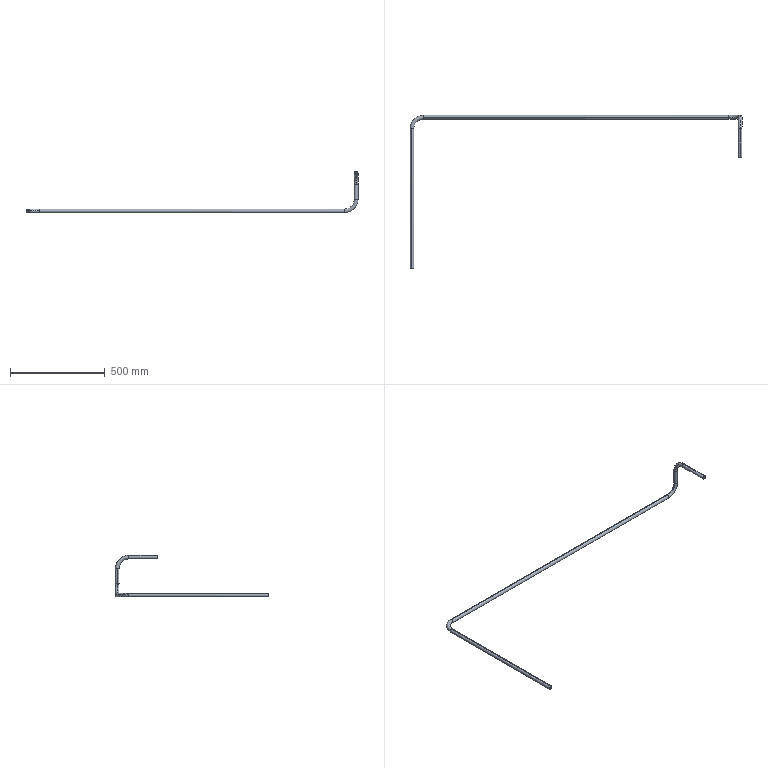Part | SolidWorks | features 3DProfileFeature 2, Sweep 1 | 1 solid | 30 faces | box 1755 x 810 x 220 mm | volume 676261 mm3 | cylinder 16 | torus 12 | plane 2 | commonest cylinder face diameters 10 x8 20 x8
STEP:
#1=CARTESIAN_POINT('',(725.349,1850.038,-1305.));
#2=VERTEX_POINT('',#1);
#3=CARTESIAN_POINT('',(725.349,1855.038,-1300.));
#4=VERTEX_POINT('',#3);
#5=CARTESIAN_POINT('',(725.349,1850.038,-1300.));
#6=DIRECTION('',(1.,0.,0.));
#7=DIRECTION('',(0.,0.,1.));
#8=AXIS2_PLACEMENT_3D('',#5,#6,#7);
#9=CIRCLE('',#8,5.);
#10=EDGE_CURVE('',#2,#4,#9,.T.);
#11=ORIENTED_EDGE('',*,*,#10,.T.);
#12=CARTESIAN_POINT('',(660.349,1790.038,-1300.));
#13=VERTEX_POINT('',#12);
#14=CARTESIAN_POINT('',(725.349,1790.038,-1300.));
#15=DIRECTION('',(0.,0.,1.));
#16=DIRECTION('',(1.,0.,0.));
#17=AXIS2_PLACEMENT_3D('',#14,#15,#16);
#18=CIRCLE('',#17,65.);
#19=EDGE_CURVE('',#4,#13,#18,.T.);
#20=ORIENTED_EDGE('',*,*,#19,.T.);
#21=CARTESIAN_POINT('',(665.349,1790.038,-1305.));
#22=VERTEX_POINT('',#21);
#23=CARTESIAN_POINT('',(665.349,1790.038,-1300.));
#24=DIRECTION('',(0.,1.,0.));
#25=DIRECTION('',(-1.,0.,0.));
#26=AXIS2_PLACEMENT_3D('',#23,#24,#25);
#27=CIRCLE('',#26,5.);
#28=EDGE_CURVE('',#22,#13,#27,.T.);
#29=ORIENTED_EDGE('',*,*,#28,.F.);
#30=CARTESIAN_POINT('',(670.349,1790.038,-1300.));
#31=VERTEX_POINT('',#30);
#32=CARTESIAN_POINT('',(665.349,1790.038,-1300.));
#33=DIRECTION('',(0.,1.,0.));
#34=DIRECTION('',(-1.,0.,0.));
#35=AXIS2_PLACEMENT_3D('',#32,#33,#34);
#36=CIRCLE('',#35,5.);
#37=EDGE_CURVE('',#31,#22,#36,.T.);
#38=ORIENTED_EDGE('',*,*,#37,.F.);
#39=CARTESIAN_POINT('',(725.349,1845.038,-1300.));
#40=VERTEX_POINT('',#39);
#41=CARTESIAN_POINT('',(725.349,1790.038,-1300.));
#42=DIRECTION('',(0.,0.,1.));
#43=DIRECTION('',(1.,0.,0.));
#44=AXIS2_PLACEMENT_3D('',#41,#42,#43);
#45=CIRCLE('',#44,55.);
#46=EDGE_CURVE('',#40,#31,#45,.T.);
#47=ORIENTED_EDGE('',*,*,#46,.F.);
#48=CARTESIAN_POINT('',(725.349,1850.038,-1300.));
#49=DIRECTION('',(1.,0.,0.));
#50=DIRECTION('',(0.,0.,1.));
#51=AXIS2_PLACEMENT_3D('',#48,#49,#50);
#52=CIRCLE('',#51,5.);
#53=EDGE_CURVE('',#40,#2,#52,.T.);
#54=ORIENTED_EDGE('',*,*,#53,.T.);
#55=EDGE_LOOP('',(#11,#20,#29,#38,#47,#54));
#56=FACE_OUTER_BOUND('',#55,.T.);
#57=CARTESIAN_POINT('',(725.349,1790.038,-1300.));
#58=DIRECTION('',(0.,0.,1.));
#59=DIRECTION('',(1.,0.,0.));
#60=AXIS2_PLACEMENT_3D('',#57,#58,#59);
#61=TOROIDAL_SURFACE('',#60,60.,5.);
#62=ADVANCED_FACE('',(#56),#61,.F.);
#63=CARTESIAN_POINT('',(2395.,1850.038,-1240.));
#64=VERTEX_POINT('',#63);
#65=CARTESIAN_POINT('',(2405.,1850.038,-1240.));
#66=VERTEX_POINT('',#65);
#67=CARTESIAN_POINT('',(2400.,1850.038,-1240.));
#68=DIRECTION('',(0.,0.,1.));
#69=DIRECTION('',(-1.,0.,0.));
#70=AXIS2_PLACEMENT_3D('',#67,#68,#69);
#71=CIRCLE('',#70,5.);
#72=EDGE_CURVE('',#64,#66,#71,.T.);
#73=ORIENTED_EDGE('',*,*,#72,.T.);
#74=CARTESIAN_POINT('',(2340.,1850.038,-1305.));
#75=VERTEX_POINT('',#74);
#76=CARTESIAN_POINT('',(2340.,1850.038,-1240.));
#77=DIRECTION('',(0.,1.,0.));
#78=DIRECTION('',(0.,0.,1.));
#79=AXIS2_PLACEMENT_3D('',#76,#77,#78);
#80=CIRCLE('',#79,65.);
#81=EDGE_CURVE('',#66,#75,#80,.T.);
#82=ORIENTED_EDGE('',*,*,#81,.T.);
#83=CARTESIAN_POINT('',(2340.,1850.038,-1295.));
#84=VERTEX_POINT('',#83);
#85=CARTESIAN_POINT('',(2340.,1850.038,-1300.));
#86=DIRECTION('',(1.,0.,0.));
#87=DIRECTION('',(0.,0.,-1.));
#88=AXIS2_PLACEMENT_3D('',#85,#86,#87);
#89=CIRCLE('',#88,5.);
#90=EDGE_CURVE('',#84,#75,#89,.T.);
#91=ORIENTED_EDGE('',*,*,#90,.F.);
#92=CARTESIAN_POINT('',(2340.,1850.038,-1240.));
#93=DIRECTION('',(0.,1.,0.));
#94=DIRECTION('',(0.,0.,1.));
#95=AXIS2_PLACEMENT_3D('',#92,#93,#94);
#96=CIRCLE('',#95,55.);
#97=EDGE_CURVE('',#64,#84,#96,.T.);
#98=ORIENTED_EDGE('',*,*,#97,.F.);
#99=EDGE_LOOP('',(#73,#82,#91,#98));
#100=FACE_OUTER_BOUND('',#99,.T.);
#101=CARTESIAN_POINT('',(2340.,1850.038,-1240.));
#102=DIRECTION('',(0.,1.,0.));
#103=DIRECTION('',(0.,0.,1.));
#104=AXIS2_PLACEMENT_3D('',#101,#102,#103);
#105=TOROIDAL_SURFACE('',#104,60.,5.);
#106=ADVANCED_FACE('',(#100),#105,.F.);
#107=CARTESIAN_POINT('',(2400.,1790.038,-1105.));
#108=VERTEX_POINT('',#107);
#109=CARTESIAN_POINT('',(2400.,1790.038,-1095.));
#110=VERTEX_POINT('',#109);
#111=CARTESIAN_POINT('',(2400.,1790.038,-1100.));
#112=DIRECTION('',(0.,-1.,0.));
#113=DIRECTION('',(0.,0.,1.));
#114=AXIS2_PLACEMENT_3D('',#111,#112,#113);
#115=CIRCLE('',#114,5.);
#116=EDGE_CURVE('',#108,#110,#115,.T.);
#117=ORIENTED_EDGE('',*,*,#116,.T.);
#118=CARTESIAN_POINT('',(2400.,1855.038,-1160.));
#119=VERTEX_POINT('',#118);
#120=CARTESIAN_POINT('',(2400.,1790.038,-1160.));
#121=DIRECTION('',(-1.,0.,0.));
#122=DIRECTION('',(0.,0.,1.));
#123=AXIS2_PLACEMENT_3D('',#120,#121,#122);
#124=CIRCLE('',#123,65.);
#125=EDGE_CURVE('',#110,#119,#124,.T.);
#126=ORIENTED_EDGE('',*,*,#125,.T.);
#127=CARTESIAN_POINT('',(2405.,1850.038,-1160.));
#128=VERTEX_POINT('',#127);
#129=CARTESIAN_POINT('',(2400.,1850.038,-1160.));
#130=DIRECTION('',(0.,0.,1.));
#131=DIRECTION('',(0.,-1.,0.));
#132=AXIS2_PLACEMENT_3D('',#129,#130,#131);
#133=CIRCLE('',#132,5.);
#134=EDGE_CURVE('',#128,#119,#133,.T.);
#135=ORIENTED_EDGE('',*,*,#134,.F.);
#136=CARTESIAN_POINT('',(2400.,1845.038,-1160.));
#137=VERTEX_POINT('',#136);
#138=CARTESIAN_POINT('',(2400.,1850.038,-1160.));
#139=DIRECTION('',(0.,0.,1.));
#140=DIRECTION('',(0.,-1.,0.));
#141=AXIS2_PLACEMENT_3D('',#138,#139,#140);
#142=CIRCLE('',#141,5.);
#143=EDGE_CURVE('',#137,#128,#142,.T.);
#144=ORIENTED_EDGE('',*,*,#143,.F.);
#145=CARTESIAN_POINT('',(2400.,1790.038,-1160.));
#146=DIRECTION('',(-1.,0.,0.));
#147=DIRECTION('',(0.,0.,1.));
#148=AXIS2_PLACEMENT_3D('',#145,#146,#147);
#149=CIRCLE('',#148,55.);
#150=EDGE_CURVE('',#108,#137,#149,.T.);
#151=ORIENTED_EDGE('',*,*,#150,.F.);
#152=EDGE_LOOP('',(#117,#126,#135,#144,#151));
#153=FACE_OUTER_BOUND('',#152,.T.);
#154=CARTESIAN_POINT('',(2400.,1790.038,-1160.));
#155=DIRECTION('',(-1.,0.,0.));
#156=DIRECTION('',(0.,0.,1.));
#157=AXIS2_PLACEMENT_3D('',#154,#155,#156);
#158=TOROIDAL_SURFACE('',#157,60.,5.);
#159=ADVANCED_FACE('',(#153),#158,.F.);
#160=CARTESIAN_POINT('',(725.349,1860.038,-1300.));
#161=VERTEX_POINT('',#160);
#162=CARTESIAN_POINT('',(725.349,1850.038,-1290.));
#163=VERTEX_POINT('',#162);
#164=CARTESIAN_POINT('',(725.349,1850.038,-1300.));
#165=DIRECTION('',(1.,0.,0.));
#166=DIRECTION('',(0.,0.,1.));
#167=AXIS2_PLACEMENT_3D('',#164,#165,#166);
#168=CIRCLE('',#167,10.);
#169=EDGE_CURVE('',#161,#163,#168,.T.);
#170=ORIENTED_EDGE('',*,*,#169,.F.);
#171=CARTESIAN_POINT('',(655.349,1790.038,-1300.));
#172=VERTEX_POINT('',#171);
#173=CARTESIAN_POINT('',(725.349,1790.038,-1300.));
#174=DIRECTION('',(0.,0.,1.));
#175=DIRECTION('',(1.,0.,0.));
#176=AXIS2_PLACEMENT_3D('',#173,#174,#175);
#177=CIRCLE('',#176,70.);
#178=EDGE_CURVE('',#161,#172,#177,.T.);
#179=ORIENTED_EDGE('',*,*,#178,.T.);
#180=CARTESIAN_POINT('',(665.349,1790.038,-1290.));
#181=VERTEX_POINT('',#180);
#182=CARTESIAN_POINT('',(665.349,1790.038,-1300.));
#183=DIRECTION('',(0.,1.,0.));
#184=DIRECTION('',(0.,0.,1.));
#185=AXIS2_PLACEMENT_3D('',#182,#183,#184);
#186=CIRCLE('',#185,10.);
#187=EDGE_CURVE('',#172,#181,#186,.T.);
#188=ORIENTED_EDGE('',*,*,#187,.T.);
#189=CARTESIAN_POINT('',(675.349,1790.038,-1300.));
#190=VERTEX_POINT('',#189);
#191=CARTESIAN_POINT('',(665.349,1790.038,-1300.));
#192=DIRECTION('',(0.,1.,0.));
#193=DIRECTION('',(0.,0.,1.));
#194=AXIS2_PLACEMENT_3D('',#191,#192,#193);
#195=CIRCLE('',#194,10.);
#196=EDGE_CURVE('',#181,#190,#195,.T.);
#197=ORIENTED_EDGE('',*,*,#196,.T.);
#198=CARTESIAN_POINT('',(725.349,1840.038,-1300.));
#199=VERTEX_POINT('',#198);
#200=CARTESIAN_POINT('',(725.349,1790.038,-1300.));
#201=DIRECTION('',(0.,0.,1.));
#202=DIRECTION('',(1.,0.,0.));
#203=AXIS2_PLACEMENT_3D('',#200,#201,#202);
#204=CIRCLE('',#203,50.);
#205=EDGE_CURVE('',#199,#190,#204,.T.);
#206=ORIENTED_EDGE('',*,*,#205,.F.);
#207=CARTESIAN_POINT('',(725.349,1850.038,-1300.));
#208=DIRECTION('',(1.,0.,0.));
#209=DIRECTION('',(0.,0.,1.));
#210=AXIS2_PLACEMENT_3D('',#207,#208,#209);
#211=CIRCLE('',#210,10.);
#212=EDGE_CURVE('',#163,#199,#211,.T.);
#213=ORIENTED_EDGE('',*,*,#212,.F.);
#214=EDGE_LOOP('',(#170,#179,#188,#197,#206,#213));
#215=FACE_OUTER_BOUND('',#214,.T.);
#216=CARTESIAN_POINT('',(725.349,1790.038,-1300.));
#217=DIRECTION('',(0.,0.,1.));
#218=DIRECTION('',(1.,0.,0.));
#219=AXIS2_PLACEMENT_3D('',#216,#217,#218);
#220=TOROIDAL_SURFACE('',#219,60.,10.);
#221=ADVANCED_FACE('',(#215),#220,.T.);
#222=CARTESIAN_POINT('',(2410.,1850.038,-1240.));
#223=VERTEX_POINT('',#222);
#224=CARTESIAN_POINT('',(2390.,1850.038,-1240.));
#225=VERTEX_POINT('',#224);
#226=CARTESIAN_POINT('',(2400.,1850.038,-1240.));
#227=DIRECTION('',(0.,0.,1.));
#228=DIRECTION('',(-1.,0.,0.));
#229=AXIS2_PLACEMENT_3D('',#226,#227,#228);
#230=CIRCLE('',#229,10.);
#231=EDGE_CURVE('',#223,#225,#230,.T.);
#232=ORIENTED_EDGE('',*,*,#231,.F.);
#233=CARTESIAN_POINT('',(2340.,1850.038,-1310.));
#234=VERTEX_POINT('',#233);
#235=CARTESIAN_POINT('',(2340.,1850.038,-1240.));
#236=DIRECTION('',(0.,1.,0.));
#237=DIRECTION('',(0.,0.,1.));
#238=AXIS2_PLACEMENT_3D('',#235,#236,#237);
#239=CIRCLE('',#238,70.);
#240=EDGE_CURVE('',#223,#234,#239,.T.);
#241=ORIENTED_EDGE('',*,*,#240,.T.);
#242=CARTESIAN_POINT('',(2340.,1850.038,-1290.));
#243=VERTEX_POINT('',#242);
#244=CARTESIAN_POINT('',(2340.,1850.038,-1300.));
#245=DIRECTION('',(1.,0.,0.));
#246=DIRECTION('',(0.,0.,1.));
#247=AXIS2_PLACEMENT_3D('',#244,#245,#246);
#248=CIRCLE('',#247,10.);
#249=EDGE_CURVE('',#234,#243,#248,.T.);
#250=ORIENTED_EDGE('',*,*,#249,.T.);
#251=CARTESIAN_POINT('',(2340.,1850.038,-1240.));
#252=DIRECTION('',(0.,1.,0.));
#253=DIRECTION('',(0.,0.,1.));
#254=AXIS2_PLACEMENT_3D('',#251,#252,#253);
#255=CIRCLE('',#254,50.);
#256=EDGE_CURVE('',#225,#243,#255,.T.);
#257=ORIENTED_EDGE('',*,*,#256,.F.);
#258=EDGE_LOOP('',(#232,#241,#250,#257));
#259=FACE_OUTER_BOUND('',#258,.T.);
#260=CARTESIAN_POINT('',(2340.,1850.038,-1240.));
#261=DIRECTION('',(0.,1.,0.));
#262=DIRECTION('',(0.,0.,1.));
#263=AXIS2_PLACEMENT_3D('',#260,#261,#262);
#264=TOROIDAL_SURFACE('',#263,60.,10.);
#265=ADVANCED_FACE('',(#259),#264,.T.);
#266=CARTESIAN_POINT('',(2400.,1790.038,-1090.));
#267=VERTEX_POINT('',#266);
#268=CARTESIAN_POINT('',(2400.,1790.038,-1110.));
#269=VERTEX_POINT('',#268);
#270=CARTESIAN_POINT('',(2400.,1790.038,-1100.));
#271=DIRECTION('',(0.,-1.,0.));
#272=DIRECTION('',(-1.,0.,0.));
#273=AXIS2_PLACEMENT_3D('',#270,#271,#272);
#274=CIRCLE('',#273,10.);
#275=EDGE_CURVE('',#267,#269,#274,.T.);
#276=ORIENTED_EDGE('',*,*,#275,.F.);
#277=CARTESIAN_POINT('',(2400.,1860.038,-1160.));
#278=VERTEX_POINT('',#277);
#279=CARTESIAN_POINT('',(2400.,1790.038,-1160.));
#280=DIRECTION('',(-1.,0.,0.));
#281=DIRECTION('',(0.,0.,1.));
#282=AXIS2_PLACEMENT_3D('',#279,#280,#281);
#283=CIRCLE('',#282,70.);
#284=EDGE_CURVE('',#267,#278,#283,.T.);
#285=ORIENTED_EDGE('',*,*,#284,.T.);
#286=CARTESIAN_POINT('',(2390.,1850.038,-1160.));
#287=VERTEX_POINT('',#286);
#288=CARTESIAN_POINT('',(2400.,1850.038,-1160.));
#289=DIRECTION('',(0.,0.,1.));
#290=DIRECTION('',(-1.,0.,0.));
#291=AXIS2_PLACEMENT_3D('',#288,#289,#290);
#292=CIRCLE('',#291,10.);
#293=EDGE_CURVE('',#278,#287,#292,.T.);
#294=ORIENTED_EDGE('',*,*,#293,.T.);
#295=CARTESIAN_POINT('',(2400.,1840.038,-1160.));
#296=VERTEX_POINT('',#295);
#297=CARTESIAN_POINT('',(2400.,1850.038,-1160.));
#298=DIRECTION('',(0.,0.,1.));
#299=DIRECTION('',(-1.,0.,0.));
#300=AXIS2_PLACEMENT_3D('',#297,#298,#299);
#301=CIRCLE('',#300,10.);
#302=EDGE_CURVE('',#287,#296,#301,.T.);
#303=ORIENTED_EDGE('',*,*,#302,.T.);
#304=CARTESIAN_POINT('',(2400.,1790.038,-1160.));
#305=DIRECTION('',(-1.,0.,0.));
#306=DIRECTION('',(0.,0.,1.));
#307=AXIS2_PLACEMENT_3D('',#304,#305,#306);
#308=CIRCLE('',#307,50.);
#309=EDGE_CURVE('',#269,#296,#308,.T.);
#310=ORIENTED_EDGE('',*,*,#309,.F.);
#311=EDGE_LOOP('',(#276,#285,#294,#303,#310));
#312=FACE_OUTER_BOUND('',#311,.T.);
#313=CARTESIAN_POINT('',(2400.,1790.038,-1160.));
#314=DIRECTION('',(-1.,0.,0.));
#315=DIRECTION('',(0.,0.,1.));
#316=AXIS2_PLACEMENT_3D('',#313,#314,#315);
#317=TOROIDAL_SURFACE('',#316,60.,10.);
#318=ADVANCED_FACE('',(#312),#317,.T.);
#319=ORIENTED_EDGE('',*,*,#28,.T.);
#320=CARTESIAN_POINT('',(665.349,1790.038,-1295.));
#321=VERTEX_POINT('',#320);
#322=CARTESIAN_POINT('',(665.349,1790.038,-1300.));
#323=DIRECTION('',(0.,1.,0.));
#324=DIRECTION('',(-1.,0.,0.));
#325=AXIS2_PLACEMENT_3D('',#322,#323,#324);
#326=CIRCLE('',#325,5.);
#327=EDGE_CURVE('',#13,#321,#326,.T.);
#328=ORIENTED_EDGE('',*,*,#327,.T.);
#329=CARTESIAN_POINT('',(665.349,1050.038,-1295.));
#330=VERTEX_POINT('',#329);
#331=CARTESIAN_POINT('',(665.349,1790.038,-1295.));
#332=DIRECTION('',(0.,-1.,0.));
#333=VECTOR('',#332,1000.);
#334=LINE('',#331,#333);
#335=EDGE_CURVE('',#321,#330,#334,.T.);
#336=ORIENTED_EDGE('',*,*,#335,.T.);
#337=CARTESIAN_POINT('',(665.349,1050.038,-1305.));
#338=VERTEX_POINT('',#337);
#339=CARTESIAN_POINT('',(665.349,1050.038,-1300.));
#340=DIRECTION('',(0.,1.,0.));
#341=DIRECTION('',(0.,0.,1.));
#342=AXIS2_PLACEMENT_3D('',#339,#340,#341);
#343=CIRCLE('',#342,5.);
#344=EDGE_CURVE('',#338,#330,#343,.T.);
#345=ORIENTED_EDGE('',*,*,#344,.F.);
#346=CARTESIAN_POINT('',(665.349,1790.038,-1305.));
#347=DIRECTION('',(0.,-1.,0.));
#348=VECTOR('',#347,1000.);
#349=LINE('',#346,#348);
#350=EDGE_CURVE('',#22,#338,#349,.T.);
#351=ORIENTED_EDGE('',*,*,#350,.F.);
#352=EDGE_LOOP('',(#319,#328,#336,#345,#351));
#353=FACE_OUTER_BOUND('',#352,.T.);
#354=CARTESIAN_POINT('',(665.349,1790.038,-1300.));
#355=DIRECTION('',(0.,-1.,0.));
#356=DIRECTION('',(0.,0.,-1.));
#357=AXIS2_PLACEMENT_3D('',#354,#355,#356);
#358=CYLINDRICAL_SURFACE('',#357,5.);
#359=ADVANCED_FACE('',(#353),#358,.F.);
#360=ORIENTED_EDGE('',*,*,#90,.T.);
#361=CARTESIAN_POINT('',(2340.,1850.038,-1305.));
#362=DIRECTION('',(-1.,0.,0.));
#363=VECTOR('',#362,1000.);
#364=LINE('',#361,#363);
#365=EDGE_CURVE('',#75,#2,#364,.T.);
#366=ORIENTED_EDGE('',*,*,#365,.T.);
#367=ORIENTED_EDGE('',*,*,#53,.F.);
#368=CARTESIAN_POINT('',(725.349,1850.038,-1295.));
#369=VERTEX_POINT('',#368);
#370=CARTESIAN_POINT('',(725.349,1850.038,-1300.));
#371=DIRECTION('',(1.,0.,0.));
#372=DIRECTION('',(0.,0.,1.));
#373=AXIS2_PLACEMENT_3D('',#370,#371,#372);
#374=CIRCLE('',#373,5.);
#375=EDGE_CURVE('',#369,#40,#374,.T.);
#376=ORIENTED_EDGE('',*,*,#375,.F.);
#377=CARTESIAN_POINT('',(2340.,1850.038,-1295.));
#378=DIRECTION('',(-1.,0.,0.));
#379=VECTOR('',#378,1000.);
#380=LINE('',#377,#379);
#381=EDGE_CURVE('',#84,#369,#380,.T.);
#382=ORIENTED_EDGE('',*,*,#381,.F.);
#383=EDGE_LOOP('',(#360,#366,#367,#376,#382));
#384=FACE_OUTER_BOUND('',#383,.T.);
#385=CARTESIAN_POINT('',(2340.,1850.038,-1300.));
#386=DIRECTION('',(-1.,0.,0.));
#387=DIRECTION('',(0.,0.,1.));
#388=AXIS2_PLACEMENT_3D('',#385,#386,#387);
#389=CYLINDRICAL_SURFACE('',#388,5.);
#390=ADVANCED_FACE('',(#384),#389,.F.);
#391=CARTESIAN_POINT('',(2395.,1850.038,-1160.));
#392=VERTEX_POINT('',#391);
#393=CARTESIAN_POINT('',(2400.,1850.038,-1160.));
#394=DIRECTION('',(0.,0.,1.));
#395=DIRECTION('',(0.,-1.,0.));
#396=AXIS2_PLACEMENT_3D('',#393,#394,#395);
#397=CIRCLE('',#396,5.);
#398=EDGE_CURVE('',#392,#137,#397,.T.);
#399=ORIENTED_EDGE('',*,*,#398,.T.);
#400=ORIENTED_EDGE('',*,*,#143,.T.);
#401=CARTESIAN_POINT('',(2405.,1850.038,-1160.));
#402=DIRECTION('',(0.,0.,-1.));
#403=VECTOR('',#402,1000.);
#404=LINE('',#401,#403);
#405=EDGE_CURVE('',#128,#66,#404,.T.);
#406=ORIENTED_EDGE('',*,*,#405,.T.);
#407=ORIENTED_EDGE('',*,*,#72,.F.);
#408=CARTESIAN_POINT('',(2395.,1850.038,-1160.));
#409=DIRECTION('',(0.,0.,-1.));
#410=VECTOR('',#409,1000.);
#411=LINE('',#408,#410);
#412=EDGE_CURVE('',#392,#64,#411,.T.);
#413=ORIENTED_EDGE('',*,*,#412,.F.);
#414=EDGE_LOOP('',(#399,#400,#406,#407,#413));
#415=FACE_OUTER_BOUND('',#414,.T.);
#416=CARTESIAN_POINT('',(2400.,1850.038,-1160.));
#417=DIRECTION('',(0.,0.,-1.));
#418=DIRECTION('',(-1.,0.,0.));
#419=AXIS2_PLACEMENT_3D('',#416,#417,#418);
#420=CYLINDRICAL_SURFACE('',#419,5.);
#421=ADVANCED_FACE('',(#415),#420,.F.);
#422=CARTESIAN_POINT('',(2400.,1637.292,-1095.));
#423=VERTEX_POINT('',#422);
#424=CARTESIAN_POINT('',(2400.,1637.292,-1105.));
#425=VERTEX_POINT('',#424);
#426=CARTESIAN_POINT('',(2400.,1637.292,-1100.));
#427=DIRECTION('',(0.,-1.,0.));
#428=DIRECTION('',(0.,0.,-1.));
#429=AXIS2_PLACEMENT_3D('',#426,#427,#428);
#430=CIRCLE('',#429,5.);
#431=EDGE_CURVE('',#423,#425,#430,.T.);
#432=ORIENTED_EDGE('',*,*,#431,.T.);
#433=CARTESIAN_POINT('',(2400.,1637.292,-1105.));
#434=DIRECTION('',(0.,1.,0.));
#435=VECTOR('',#434,1000.);
#436=LINE('',#433,#435);
#437=EDGE_CURVE('',#425,#108,#436,.T.);
#438=ORIENTED_EDGE('',*,*,#437,.T.);
#439=CARTESIAN_POINT('',(2400.,1790.038,-1100.));
#440=DIRECTION('',(0.,-1.,0.));
#441=DIRECTION('',(0.,0.,1.));
#442=AXIS2_PLACEMENT_3D('',#439,#440,#441);
#443=CIRCLE('',#442,5.);
#444=EDGE_CURVE('',#110,#108,#443,.T.);
#445=ORIENTED_EDGE('',*,*,#444,.F.);
#446=CARTESIAN_POINT('',(2400.,1637.292,-1095.));
#447=DIRECTION('',(0.,1.,0.));
#448=VECTOR('',#447,1000.);
#449=LINE('',#446,#448);
#450=EDGE_CURVE('',#423,#110,#449,.T.);
#451=ORIENTED_EDGE('',*,*,#450,.F.);
#452=EDGE_LOOP('',(#432,#438,#445,#451));
#453=FACE_OUTER_BOUND('',#452,.T.);
#454=CARTESIAN_POINT('',(2400.,1637.292,-1100.));
#455=DIRECTION('',(0.,1.,0.));
#456=DIRECTION('',(0.,0.,1.));
#457=AXIS2_PLACEMENT_3D('',#454,#455,#456);
#458=CYLINDRICAL_SURFACE('',#457,5.);
#459=ADVANCED_FACE('',(#453),#458,.F.);
#460=ORIENTED_EDGE('',*,*,#196,.F.);
#461=CARTESIAN_POINT('',(665.349,1050.038,-1290.));
#462=VERTEX_POINT('',#461);
#463=CARTESIAN_POINT('',(665.349,1790.038,-1290.));
#464=DIRECTION('',(0.,-1.,0.));
#465=VECTOR('',#464,1000.);
#466=LINE('',#463,#465);
#467=EDGE_CURVE('',#181,#462,#466,.T.);
#468=ORIENTED_EDGE('',*,*,#467,.T.);
#469=CARTESIAN_POINT('',(665.349,1050.038,-1310.));
#470=VERTEX_POINT('',#469);
#471=CARTESIAN_POINT('',(665.349,1050.038,-1300.));
#472=DIRECTION('',(0.,1.,0.));
#473=DIRECTION('',(0.,0.,1.));
#474=AXIS2_PLACEMENT_3D('',#471,#472,#473);
#475=CIRCLE('',#474,10.);
#476=EDGE_CURVE('',#462,#470,#475,.T.);
#477=ORIENTED_EDGE('',*,*,#476,.T.);
#478=CARTESIAN_POINT('',(665.349,1790.038,-1310.));
#479=VERTEX_POINT('',#478);
#480=CARTESIAN_POINT('',(665.349,1790.038,-1310.));
#481=DIRECTION('',(0.,-1.,0.));
#482=VECTOR('',#481,1000.);
#483=LINE('',#480,#482);
#484=EDGE_CURVE('',#479,#470,#483,.T.);
#485=ORIENTED_EDGE('',*,*,#484,.F.);
#486=CARTESIAN_POINT('',(665.349,1790.038,-1300.));
#487=DIRECTION('',(0.,1.,0.));
#488=DIRECTION('',(0.,0.,1.));
#489=AXIS2_PLACEMENT_3D('',#486,#487,#488);
#490=CIRCLE('',#489,10.);
#491=EDGE_CURVE('',#190,#479,#490,.T.);
#492=ORIENTED_EDGE('',*,*,#491,.F.);
#493=EDGE_LOOP('',(#460,#468,#477,#485,#492));
#494=FACE_OUTER_BOUND('',#493,.T.);
#495=CARTESIAN_POINT('',(665.349,1790.038,-1300.));
#496=DIRECTION('',(0.,-1.,0.));
#497=DIRECTION('',(0.,0.,-1.));
#498=AXIS2_PLACEMENT_3D('',#495,#496,#497);
#499=CYLINDRICAL_SURFACE('',#498,10.);
#500=ADVANCED_FACE('',(#494),#499,.T.);
#501=ORIENTED_EDGE('',*,*,#249,.F.);
#502=CARTESIAN_POINT('',(725.349,1850.038,-1310.));
#503=VERTEX_POINT('',#502);
#504=CARTESIAN_POINT('',(2340.,1850.038,-1310.));
#505=DIRECTION('',(-1.,0.,0.));
#506=VECTOR('',#505,1000.);
#507=LINE('',#504,#506);
#508=EDGE_CURVE('',#234,#503,#507,.T.);
#509=ORIENTED_EDGE('',*,*,#508,.T.);
#510=CARTESIAN_POINT('',(725.349,1850.038,-1300.));
#511=DIRECTION('',(1.,0.,0.));
#512=DIRECTION('',(0.,0.,1.));
#513=AXIS2_PLACEMENT_3D('',#510,#511,#512);
#514=CIRCLE('',#513,10.);
#515=EDGE_CURVE('',#503,#161,#514,.T.);
#516=ORIENTED_EDGE('',*,*,#515,.T.);
#517=ORIENTED_EDGE('',*,*,#169,.T.);
#518=CARTESIAN_POINT('',(2340.,1850.038,-1290.));
#519=DIRECTION('',(-1.,0.,0.));
#520=VECTOR('',#519,1000.);
#521=LINE('',#518,#520);
#522=EDGE_CURVE('',#243,#163,#521,.T.);
#523=ORIENTED_EDGE('',*,*,#522,.F.);
#524=EDGE_LOOP('',(#501,#509,#516,#517,#523));
#525=FACE_OUTER_BOUND('',#524,.T.);
#526=CARTESIAN_POINT('',(2340.,1850.038,-1300.));
#527=DIRECTION('',(-1.,0.,0.));
#528=DIRECTION('',(0.,0.,1.));
#529=AXIS2_PLACEMENT_3D('',#526,#527,#528);
#530=CYLINDRICAL_SURFACE('',#529,10.);
#531=ADVANCED_FACE('',(#525),#530,.T.);
#532=CARTESIAN_POINT('',(2410.,1850.038,-1160.));
#533=VERTEX_POINT('',#532);
#534=CARTESIAN_POINT('',(2400.,1850.038,-1160.));
#535=DIRECTION('',(0.,0.,1.));
#536=DIRECTION('',(-1.,0.,0.));
#537=AXIS2_PLACEMENT_3D('',#534,#535,#536);
#538=CIRCLE('',#537,10.);
#539=EDGE_CURVE('',#533,#278,#538,.T.);
#540=ORIENTED_EDGE('',*,*,#539,.F.);
#541=CARTESIAN_POINT('',(2410.,1850.038,-1160.));
#542=DIRECTION('',(0.,0.,-1.));
#543=VECTOR('',#542,1000.);
#544=LINE('',#541,#543);
#545=EDGE_CURVE('',#533,#223,#544,.T.);
#546=ORIENTED_EDGE('',*,*,#545,.T.);
#547=ORIENTED_EDGE('',*,*,#231,.T.);
#548=CARTESIAN_POINT('',(2390.,1850.038,-1160.));
#549=DIRECTION('',(0.,0.,-1.));
#550=VECTOR('',#549,1000.);
#551=LINE('',#548,#550);
#552=EDGE_CURVE('',#287,#225,#551,.T.);
#553=ORIENTED_EDGE('',*,*,#552,.F.);
#554=ORIENTED_EDGE('',*,*,#293,.F.);
#555=EDGE_LOOP('',(#540,#546,#547,#553,#554));
#556=FACE_OUTER_BOUND('',#555,.T.);
#557=CARTESIAN_POINT('',(2400.,1850.038,-1160.));
#558=DIRECTION('',(0.,0.,-1.));
#559=DIRECTION('',(-1.,0.,0.));
#560=AXIS2_PLACEMENT_3D('',#557,#558,#559);
#561=CYLINDRICAL_SURFACE('',#560,10.);
#562=ADVANCED_FACE('',(#556),#561,.T.);
#563=CARTESIAN_POINT('',(2400.,1637.292,-1110.));
#564=VERTEX_POINT('',#563);
#565=CARTESIAN_POINT('',(2400.,1637.292,-1090.));
#566=VERTEX_POINT('',#565);
#567=CARTESIAN_POINT('',(2400.,1637.292,-1100.));
#568=DIRECTION('',(0.,-1.,0.));
#569=DIRECTION('',(-1.,0.,0.));
#570=AXIS2_PLACEMENT_3D('',#567,#568,#569);
#571=CIRCLE('',#570,10.);
#572=EDGE_CURVE('',#564,#566,#571,.T.);
#573=ORIENTED_EDGE('',*,*,#572,.F.);
#574=CARTESIAN_POINT('',(2400.,1637.292,-1110.));
#575=DIRECTION('',(0.,1.,0.));
#576=VECTOR('',#575,1000.);
#577=LINE('',#574,#576);
#578=EDGE_CURVE('',#564,#269,#577,.T.);
#579=ORIENTED_EDGE('',*,*,#578,.T.);
#580=CARTESIAN_POINT('',(2400.,1790.038,-1100.));
#581=DIRECTION('',(0.,-1.,0.));
#582=DIRECTION('',(-1.,0.,0.));
#583=AXIS2_PLACEMENT_3D('',#580,#581,#582);
#584=CIRCLE('',#583,10.);
#585=EDGE_CURVE('',#269,#267,#584,.T.);
#586=ORIENTED_EDGE('',*,*,#585,.T.);
#587=CARTESIAN_POINT('',(2400.,1637.292,-1090.));
#588=DIRECTION('',(0.,1.,0.));
#589=VECTOR('',#588,1000.);
#590=LINE('',#587,#589);
#591=EDGE_CURVE('',#566,#267,#590,.T.);
#592=ORIENTED_EDGE('',*,*,#591,.F.);
#593=EDGE_LOOP('',(#573,#579,#586,#592));
#594=FACE_OUTER_BOUND('',#593,.T.);
#595=CARTESIAN_POINT('',(2400.,1637.292,-1100.));
#596=DIRECTION('',(0.,1.,0.));
#597=DIRECTION('',(0.,0.,1.));
#598=AXIS2_PLACEMENT_3D('',#595,#596,#597);
#599=CYLINDRICAL_SURFACE('',#598,10.);
#600=ADVANCED_FACE('',(#594),#599,.T.);
#601=ORIENTED_EDGE('',*,*,#467,.F.);
#602=ORIENTED_EDGE('',*,*,#187,.F.);
#603=CARTESIAN_POINT('',(665.349,1790.038,-1300.));
#604=DIRECTION('',(0.,1.,0.));
#605=DIRECTION('',(0.,0.,1.));
#606=AXIS2_PLACEMENT_3D('',#603,#604,#605);
#607=CIRCLE('',#606,10.);
#608=EDGE_CURVE('',#479,#172,#607,.T.);
#609=ORIENTED_EDGE('',*,*,#608,.F.);
#610=ORIENTED_EDGE('',*,*,#484,.T.);
#611=CARTESIAN_POINT('',(665.349,1050.038,-1300.));
#612=DIRECTION('',(0.,1.,0.));
#613=DIRECTION('',(0.,0.,1.));
#614=AXIS2_PLACEMENT_3D('',#611,#612,#613);
#615=CIRCLE('',#614,10.);
#616=EDGE_CURVE('',#470,#462,#615,.T.);
#617=ORIENTED_EDGE('',*,*,#616,.T.);
#618=EDGE_LOOP('',(#601,#602,#609,#610,#617));
#619=FACE_OUTER_BOUND('',#618,.T.);
#620=CARTESIAN_POINT('',(665.349,1790.038,-1300.));
#621=DIRECTION('',(0.,-1.,0.));
#622=DIRECTION('',(0.,0.,-1.));
#623=AXIS2_PLACEMENT_3D('',#620,#621,#622);
#624=CYLINDRICAL_SURFACE('',#623,10.);
#625=ADVANCED_FACE('',(#619),#624,.T.);
#626=ORIENTED_EDGE('',*,*,#178,.F.);
#627=ORIENTED_EDGE('',*,*,#515,.F.);
#628=CARTESIAN_POINT('',(725.349,1850.038,-1300.));
#629=DIRECTION('',(1.,0.,0.));
#630=DIRECTION('',(0.,0.,1.));
#631=AXIS2_PLACEMENT_3D('',#628,#629,#630);
#632=CIRCLE('',#631,10.);
#633=EDGE_CURVE('',#199,#503,#632,.T.);
#634=ORIENTED_EDGE('',*,*,#633,.F.);
#635=ORIENTED_EDGE('',*,*,#205,.T.);
#636=ORIENTED_EDGE('',*,*,#491,.T.);
#637=ORIENTED_EDGE('',*,*,#608,.T.);
#638=EDGE_LOOP('',(#626,#627,#634,#635,#636,#637));
#639=FACE_OUTER_BOUND('',#638,.T.);
#640=CARTESIAN_POINT('',(725.349,1790.038,-1300.));
#641=DIRECTION('',(0.,0.,1.));
#642=DIRECTION('',(1.,0.,0.));
#643=AXIS2_PLACEMENT_3D('',#640,#641,#642);
#644=TOROIDAL_SURFACE('',#643,60.,10.);
#645=ADVANCED_FACE('',(#639),#644,.T.);
#646=ORIENTED_EDGE('',*,*,#508,.F.);
#647=CARTESIAN_POINT('',(2340.,1850.038,-1300.));
#648=DIRECTION('',(1.,0.,0.));
#649=DIRECTION('',(0.,0.,1.));
#650=AXIS2_PLACEMENT_3D('',#647,#648,#649);
#651=CIRCLE('',#650,10.);
#652=EDGE_CURVE('',#243,#234,#651,.T.);
#653=ORIENTED_EDGE('',*,*,#652,.F.);
#654=ORIENTED_EDGE('',*,*,#522,.T.);
#655=ORIENTED_EDGE('',*,*,#212,.T.);
#656=ORIENTED_EDGE('',*,*,#633,.T.);
#657=EDGE_LOOP('',(#646,#653,#654,#655,#656));
#658=FACE_OUTER_BOUND('',#657,.T.);
#659=CARTESIAN_POINT('',(2340.,1850.038,-1300.));
#660=DIRECTION('',(-1.,0.,0.));
#661=DIRECTION('',(0.,0.,1.));
#662=AXIS2_PLACEMENT_3D('',#659,#660,#661);
#663=CYLINDRICAL_SURFACE('',#662,10.);
#664=ADVANCED_FACE('',(#658),#663,.T.);
#665=ORIENTED_EDGE('',*,*,#240,.F.);
#666=CARTESIAN_POINT('',(2400.,1850.038,-1240.));
#667=DIRECTION('',(0.,0.,1.));
#668=DIRECTION('',(-1.,0.,0.));
#669=AXIS2_PLACEMENT_3D('',#666,#667,#668);
#670=CIRCLE('',#669,10.);
#671=EDGE_CURVE('',#225,#223,#670,.T.);
#672=ORIENTED_EDGE('',*,*,#671,.F.);
#673=ORIENTED_EDGE('',*,*,#256,.T.);
#674=ORIENTED_EDGE('',*,*,#652,.T.);
#675=EDGE_LOOP('',(#665,#672,#673,#674));
#676=FACE_OUTER_BOUND('',#675,.T.);
#677=CARTESIAN_POINT('',(2340.,1850.038,-1240.));
#678=DIRECTION('',(0.,1.,0.));
#679=DIRECTION('',(0.,0.,1.));
#680=AXIS2_PLACEMENT_3D('',#677,#678,#679);
#681=TOROIDAL_SURFACE('',#680,60.,10.);
#682=ADVANCED_FACE('',(#676),#681,.T.);
#683=ORIENTED_EDGE('',*,*,#545,.F.);
#684=CARTESIAN_POINT('',(2400.,1850.038,-1160.));
#685=DIRECTION('',(0.,0.,1.));
#686=DIRECTION('',(-1.,0.,0.));
#687=AXIS2_PLACEMENT_3D('',#684,#685,#686);
#688=CIRCLE('',#687,10.);
#689=EDGE_CURVE('',#296,#533,#688,.T.);
#690=ORIENTED_EDGE('',*,*,#689,.F.);
#691=ORIENTED_EDGE('',*,*,#302,.F.);
#692=ORIENTED_EDGE('',*,*,#552,.T.);
#693=ORIENTED_EDGE('',*,*,#671,.T.);
#694=EDGE_LOOP('',(#683,#690,#691,#692,#693));
#695=FACE_OUTER_BOUND('',#694,.T.);
#696=CARTESIAN_POINT('',(2400.,1850.038,-1160.));
#697=DIRECTION('',(0.,0.,-1.));
#698=DIRECTION('',(-1.,0.,0.));
#699=AXIS2_PLACEMENT_3D('',#696,#697,#698);
#700=CYLINDRICAL_SURFACE('',#699,10.);
#701=ADVANCED_FACE('',(#695),#700,.T.);
#702=ORIENTED_EDGE('',*,*,#284,.F.);
#703=ORIENTED_EDGE('',*,*,#585,.F.);
#704=ORIENTED_EDGE('',*,*,#309,.T.);
#705=ORIENTED_EDGE('',*,*,#689,.T.);
#706=ORIENTED_EDGE('',*,*,#539,.T.);
#707=EDGE_LOOP('',(#702,#703,#704,#705,#706));
#708=FACE_OUTER_BOUND('',#707,.T.);
#709=CARTESIAN_POINT('',(2400.,1790.038,-1160.));
#710=DIRECTION('',(-1.,0.,0.));
#711=DIRECTION('',(0.,0.,1.));
#712=AXIS2_PLACEMENT_3D('',#709,#710,#711);
#713=TOROIDAL_SURFACE('',#712,60.,10.);
#714=ADVANCED_FACE('',(#708),#713,.T.);
#715=ORIENTED_EDGE('',*,*,#578,.F.);
#716=CARTESIAN_POINT('',(2400.,1637.292,-1100.));
#717=DIRECTION('',(0.,-1.,0.));
#718=DIRECTION('',(-1.,0.,0.));
#719=AXIS2_PLACEMENT_3D('',#716,#717,#718);
#720=CIRCLE('',#719,10.);
#721=EDGE_CURVE('',#566,#564,#720,.T.);
#722=ORIENTED_EDGE('',*,*,#721,.F.);
#723=ORIENTED_EDGE('',*,*,#591,.T.);
#724=ORIENTED_EDGE('',*,*,#275,.T.);
#725=EDGE_LOOP('',(#715,#722,#723,#724));
#726=FACE_OUTER_BOUND('',#725,.T.);
#727=CARTESIAN_POINT('',(2400.,1637.292,-1100.));
#728=DIRECTION('',(0.,1.,0.));
#729=DIRECTION('',(0.,0.,1.));
#730=AXIS2_PLACEMENT_3D('',#727,#728,#729);
#731=CYLINDRICAL_SURFACE('',#730,10.);
#732=ADVANCED_FACE('',(#726),#731,.T.);
#733=ORIENTED_EDGE('',*,*,#344,.T.);
#734=CARTESIAN_POINT('',(665.349,1050.038,-1300.));
#735=DIRECTION('',(0.,1.,0.));
#736=DIRECTION('',(0.,0.,1.));
#737=AXIS2_PLACEMENT_3D('',#734,#735,#736);
#738=CIRCLE('',#737,5.);
#739=EDGE_CURVE('',#330,#338,#738,.T.);
#740=ORIENTED_EDGE('',*,*,#739,.T.);
#741=EDGE_LOOP('',(#733,#740));
#742=FACE_BOUND('',#741,.T.);
#743=ORIENTED_EDGE('',*,*,#616,.F.);
#744=ORIENTED_EDGE('',*,*,#476,.F.);
#745=EDGE_LOOP('',(#743,#744));
#746=FACE_OUTER_BOUND('',#745,.T.);
#747=CARTESIAN_POINT('',(665.349,1050.038,-1300.));
#748=DIRECTION('',(0.,1.,0.));
#749=DIRECTION('',(0.,0.,1.));
#750=AXIS2_PLACEMENT_3D('',#747,#748,#749);
#751=PLANE('',#750);
#752=ADVANCED_FACE('',(#742,#746),#751,.F.);
#753=ORIENTED_EDGE('',*,*,#431,.F.);
#754=CARTESIAN_POINT('',(2400.,1637.292,-1100.));
#755=DIRECTION('',(0.,-1.,0.));
#756=DIRECTION('',(0.,0.,-1.));
#757=AXIS2_PLACEMENT_3D('',#754,#755,#756);
#758=CIRCLE('',#757,5.);
#759=EDGE_CURVE('',#425,#423,#758,.T.);
#760=ORIENTED_EDGE('',*,*,#759,.F.);
#761=EDGE_LOOP('',(#753,#760));
#762=FACE_BOUND('',#761,.T.);
#763=ORIENTED_EDGE('',*,*,#721,.T.);
#764=ORIENTED_EDGE('',*,*,#572,.T.);
#765=EDGE_LOOP('',(#763,#764));
#766=FACE_OUTER_BOUND('',#765,.T.);
#767=CARTESIAN_POINT('',(2400.,1637.292,-1100.));
#768=DIRECTION('',(0.,-1.,0.));
#769=DIRECTION('',(-1.,0.,0.));
#770=AXIS2_PLACEMENT_3D('',#767,#768,#769);
#771=PLANE('',#770);
#772=ADVANCED_FACE('',(#762,#766),#771,.T.);
#773=ORIENTED_EDGE('',*,*,#335,.F.);
#774=CARTESIAN_POINT('',(665.349,1790.038,-1300.));
#775=DIRECTION('',(0.,1.,0.));
#776=DIRECTION('',(-1.,0.,0.));
#777=AXIS2_PLACEMENT_3D('',#774,#775,#776);
#778=CIRCLE('',#777,5.);
#779=EDGE_CURVE('',#321,#31,#778,.T.);
#780=ORIENTED_EDGE('',*,*,#779,.T.);
#781=ORIENTED_EDGE('',*,*,#37,.T.);
#782=ORIENTED_EDGE('',*,*,#350,.T.);
#783=ORIENTED_EDGE('',*,*,#739,.F.);
#784=EDGE_LOOP('',(#773,#780,#781,#782,#783));
#785=FACE_OUTER_BOUND('',#784,.T.);
#786=CARTESIAN_POINT('',(665.349,1790.038,-1300.));
#787=DIRECTION('',(0.,-1.,0.));
#788=DIRECTION('',(0.,0.,-1.));
#789=AXIS2_PLACEMENT_3D('',#786,#787,#788);
#790=CYLINDRICAL_SURFACE('',#789,5.);
#791=ADVANCED_FACE('',(#785),#790,.F.);
#792=ORIENTED_EDGE('',*,*,#19,.F.);
#793=CARTESIAN_POINT('',(725.349,1850.038,-1300.));
#794=DIRECTION('',(1.,0.,0.));
#795=DIRECTION('',(0.,0.,1.));
#796=AXIS2_PLACEMENT_3D('',#793,#794,#795);
#797=CIRCLE('',#796,5.);
#798=EDGE_CURVE('',#4,#369,#797,.T.);
#799=ORIENTED_EDGE('',*,*,#798,.T.);
#800=ORIENTED_EDGE('',*,*,#375,.T.);
#801=ORIENTED_EDGE('',*,*,#46,.T.);
#802=ORIENTED_EDGE('',*,*,#779,.F.);
#803=ORIENTED_EDGE('',*,*,#327,.F.);
#804=EDGE_LOOP('',(#792,#799,#800,#801,#802,#803));
#805=FACE_OUTER_BOUND('',#804,.T.);
#806=CARTESIAN_POINT('',(725.349,1790.038,-1300.));
#807=DIRECTION('',(0.,0.,1.));
#808=DIRECTION('',(1.,0.,0.));
#809=AXIS2_PLACEMENT_3D('',#806,#807,#808);
#810=TOROIDAL_SURFACE('',#809,60.,5.);
#811=ADVANCED_FACE('',(#805),#810,.F.);
#812=ORIENTED_EDGE('',*,*,#365,.F.);
#813=CARTESIAN_POINT('',(2340.,1850.038,-1300.));
#814=DIRECTION('',(1.,0.,0.));
#815=DIRECTION('',(0.,0.,-1.));
#816=AXIS2_PLACEMENT_3D('',#813,#814,#815);
#817=CIRCLE('',#816,5.);
#818=EDGE_CURVE('',#75,#84,#817,.T.);
#819=ORIENTED_EDGE('',*,*,#818,.T.);
#820=ORIENTED_EDGE('',*,*,#381,.T.);
#821=ORIENTED_EDGE('',*,*,#798,.F.);
#822=ORIENTED_EDGE('',*,*,#10,.F.);
#823=EDGE_LOOP('',(#812,#819,#820,#821,#822));
#824=FACE_OUTER_BOUND('',#823,.T.);
#825=CARTESIAN_POINT('',(2340.,1850.038,-1300.));
#826=DIRECTION('',(-1.,0.,0.));
#827=DIRECTION('',(0.,0.,1.));
#828=AXIS2_PLACEMENT_3D('',#825,#826,#827);
#829=CYLINDRICAL_SURFACE('',#828,5.);
#830=ADVANCED_FACE('',(#824),#829,.F.);
#831=ORIENTED_EDGE('',*,*,#81,.F.);
#832=CARTESIAN_POINT('',(2400.,1850.038,-1240.));
#833=DIRECTION('',(0.,0.,1.));
#834=DIRECTION('',(-1.,0.,0.));
#835=AXIS2_PLACEMENT_3D('',#832,#833,#834);
#836=CIRCLE('',#835,5.);
#837=EDGE_CURVE('',#66,#64,#836,.T.);
#838=ORIENTED_EDGE('',*,*,#837,.T.);
#839=ORIENTED_EDGE('',*,*,#97,.T.);
#840=ORIENTED_EDGE('',*,*,#818,.F.);
#841=EDGE_LOOP('',(#831,#838,#839,#840));
#842=FACE_OUTER_BOUND('',#841,.T.);
#843=CARTESIAN_POINT('',(2340.,1850.038,-1240.));
#844=DIRECTION('',(0.,1.,0.));
#845=DIRECTION('',(0.,0.,1.));
#846=AXIS2_PLACEMENT_3D('',#843,#844,#845);
#847=TOROIDAL_SURFACE('',#846,60.,5.);
#848=ADVANCED_FACE('',(#842),#847,.F.);
#849=ORIENTED_EDGE('',*,*,#405,.F.);
#850=ORIENTED_EDGE('',*,*,#134,.T.);
#851=CARTESIAN_POINT('',(2400.,1850.038,-1160.));
#852=DIRECTION('',(0.,0.,1.));
#853=DIRECTION('',(0.,-1.,0.));
#854=AXIS2_PLACEMENT_3D('',#851,#852,#853);
#855=CIRCLE('',#854,5.);
#856=EDGE_CURVE('',#119,#392,#855,.T.);
#857=ORIENTED_EDGE('',*,*,#856,.T.);
#858=ORIENTED_EDGE('',*,*,#412,.T.);
#859=ORIENTED_EDGE('',*,*,#837,.F.);
#860=EDGE_LOOP('',(#849,#850,#857,#858,#859));
#861=FACE_OUTER_BOUND('',#860,.T.);
#862=CARTESIAN_POINT('',(2400.,1850.038,-1160.));
#863=DIRECTION('',(0.,0.,-1.));
#864=DIRECTION('',(-1.,0.,0.));
#865=AXIS2_PLACEMENT_3D('',#862,#863,#864);
#866=CYLINDRICAL_SURFACE('',#865,5.);
#867=ADVANCED_FACE('',(#861),#866,.F.);
#868=ORIENTED_EDGE('',*,*,#125,.F.);
#869=ORIENTED_EDGE('',*,*,#444,.T.);
#870=ORIENTED_EDGE('',*,*,#150,.T.);
#871=ORIENTED_EDGE('',*,*,#398,.F.);
#872=ORIENTED_EDGE('',*,*,#856,.F.);
#873=EDGE_LOOP('',(#868,#869,#870,#871,#872));
#874=FACE_OUTER_BOUND('',#873,.T.);
#875=CARTESIAN_POINT('',(2400.,1790.038,-1160.));
#876=DIRECTION('',(-1.,0.,0.));
#877=DIRECTION('',(0.,0.,1.));
#878=AXIS2_PLACEMENT_3D('',#875,#876,#877);
#879=TOROIDAL_SURFACE('',#878,60.,5.);
#880=ADVANCED_FACE('',(#874),#879,.F.);
#881=ORIENTED_EDGE('',*,*,#437,.F.);
#882=ORIENTED_EDGE('',*,*,#759,.T.);
#883=ORIENTED_EDGE('',*,*,#450,.T.);
#884=ORIENTED_EDGE('',*,*,#116,.F.);
#885=EDGE_LOOP('',(#881,#882,#883,#884));
#886=FACE_OUTER_BOUND('',#885,.T.);
#887=CARTESIAN_POINT('',(2400.,1637.292,-1100.));
#888=DIRECTION('',(0.,1.,0.));
#889=DIRECTION('',(0.,0.,1.));
#890=AXIS2_PLACEMENT_3D('',#887,#888,#889);
#891=CYLINDRICAL_SURFACE('',#890,5.);
#892=ADVANCED_FACE('',(#886),#891,.F.);
#893=CLOSED_SHELL('',(#62,#106,#159,#221,#265,#318,#359,#390,#421,#459,#500,#531,#562,#600,#625,#645,#664,#682,#701,#714,#732,#752,#772,#791,#811,#830,#848,#867,#880,#892));
#894=MANIFOLD_SOLID_BREP('',#893);
#895=CARTESIAN_POINT('',(0.,0.,0.));
#896=DIRECTION('',(0.,0.,1.));
#897=DIRECTION('',(1.,0.,0.));
#898=AXIS2_PLACEMENT_3D('',#895,#896,#897);
#899=(LENGTH_UNIT()NAMED_UNIT(*)SI_UNIT(.MILLI.,.METRE.));
#900=UNCERTAINTY_MEASURE_WITH_UNIT(LENGTH_MEASURE(0.00001),#899,'','');
#901=(NAMED_UNIT(*)PLANE_ANGLE_UNIT()SI_UNIT($,.RADIAN.));
#902=(NAMED_UNIT(*)SI_UNIT($,.STERADIAN.)SOLID_ANGLE_UNIT());
#903=(GEOMETRIC_REPRESENTATION_CONTEXT(3)GLOBAL_UNCERTAINTY_ASSIGNED_CONTEXT((#900))GLOBAL_UNIT_ASSIGNED_CONTEXT((#899,#901,#902))REPRESENTATION_CONTEXT('',''));
#904=ADVANCED_BREP_SHAPE_REPRESENTATION('',(#894,#898),#903);